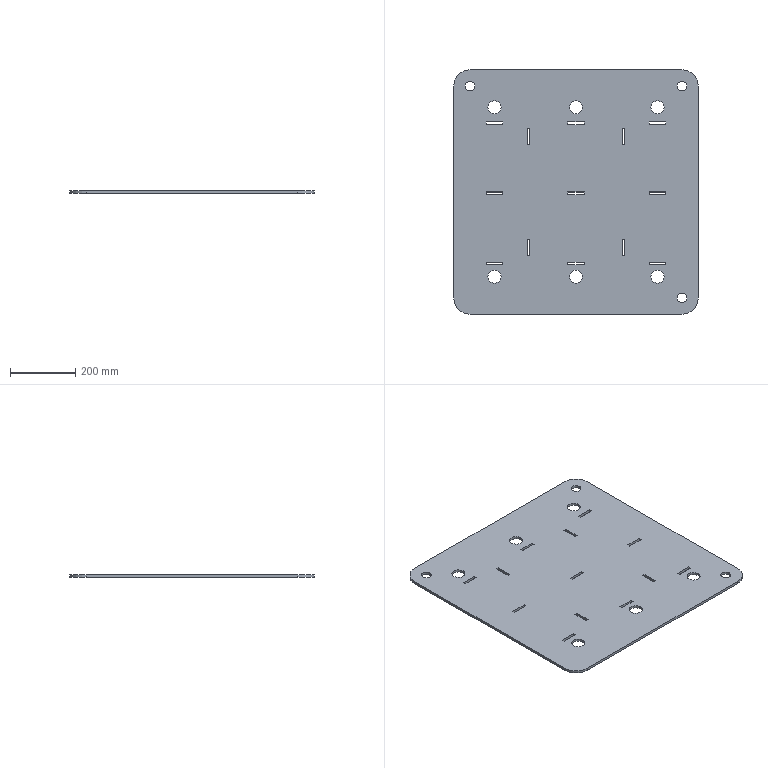Part | SolidWorks | features FlatPattern 1, ICE 1, SMBaseFlange 1, SheetMetal 1 | 1 solid | 80 faces | box 750 x 750 x 8 mm | volume 4363949 mm3 | plane 58 | cylinder 22 | commonest cylinder face diameters 40 x12 30 x6 100 x4